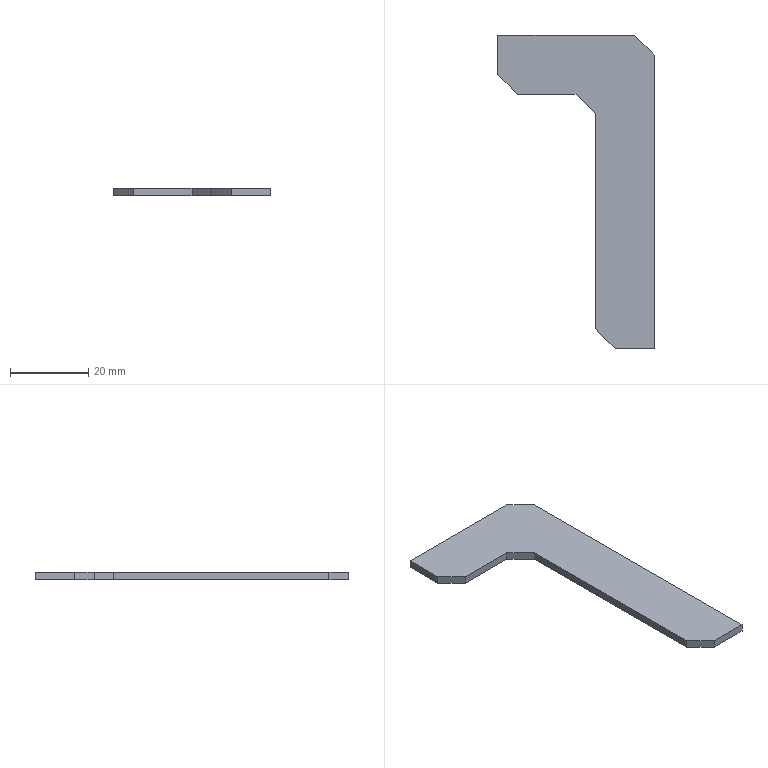Part | STEP file | SynoNew-0304-056 | 1 solid | 12 faces | box 40 x 80 x 2 mm | volume 3100 mm3 | plane 12
STEP:
#1=CARTESIAN_POINT('',(-15.,25.,2.));
#2=VERTEX_POINT('',#1);
#3=CARTESIAN_POINT('',(-20.,30.,2.));
#4=VERTEX_POINT('',#3);
#5=CARTESIAN_POINT('',(-6.25,16.25,2.));
#6=DIRECTION('',(-0.7071,0.7071,0.));
#7=VECTOR('',#6,10.);
#8=LINE('',#5,#7);
#9=EDGE_CURVE('',#2,#4,#8,.T.);
#10=ORIENTED_EDGE('',*,*,#9,.T.);
#11=CARTESIAN_POINT('',(-20.,30.,0.));
#12=VERTEX_POINT('',#11);
#13=CARTESIAN_POINT('',(-20.,30.,1.));
#14=DIRECTION('',(0.,0.,-1.));
#15=VECTOR('',#14,10.);
#16=LINE('',#13,#15);
#17=EDGE_CURVE('',#4,#12,#16,.T.);
#18=ORIENTED_EDGE('',*,*,#17,.T.);
#19=CARTESIAN_POINT('',(-15.,25.,0.));
#20=VERTEX_POINT('',#19);
#21=CARTESIAN_POINT('',(-6.25,16.25,0.));
#22=DIRECTION('',(0.7071,-0.7071,0.));
#23=VECTOR('',#22,10.);
#24=LINE('',#21,#23);
#25=EDGE_CURVE('',#12,#20,#24,.T.);
#26=ORIENTED_EDGE('',*,*,#25,.T.);
#27=CARTESIAN_POINT('',(-15.,25.,1.));
#28=DIRECTION('',(0.,0.,1.));
#29=VECTOR('',#28,10.);
#30=LINE('',#27,#29);
#31=EDGE_CURVE('',#20,#2,#30,.T.);
#32=ORIENTED_EDGE('',*,*,#31,.T.);
#33=EDGE_LOOP('',(#10,#18,#26,#32));
#34=FACE_OUTER_BOUND('',#33,.T.);
#35=CARTESIAN_POINT('',(-17.5,27.5,1.));
#36=DIRECTION('',(-0.7071,-0.7071,0.));
#37=DIRECTION('',(0.,0.,1.));
#38=AXIS2_PLACEMENT_3D('',#35,#36,#37);
#39=PLANE('',#38);
#40=ADVANCED_FACE('',(#34),#39,.T.);
#41=ORIENTED_EDGE('',*,*,#31,.F.);
#42=CARTESIAN_POINT('',(0.,25.,0.));
#43=VERTEX_POINT('',#42);
#44=CARTESIAN_POINT('',(-16.04,25.,0.));
#45=DIRECTION('',(-1.,0.,0.));
#46=VECTOR('',#45,10.);
#47=LINE('',#44,#46);
#48=EDGE_CURVE('',#43,#20,#47,.T.);
#49=ORIENTED_EDGE('',*,*,#48,.F.);
#50=CARTESIAN_POINT('',(0.,25.,2.));
#51=VERTEX_POINT('',#50);
#52=CARTESIAN_POINT('',(0.,25.,2.));
#53=DIRECTION('',(0.,0.,-1.));
#54=VECTOR('',#53,10.);
#55=LINE('',#52,#54);
#56=EDGE_CURVE('',#51,#43,#55,.T.);
#57=ORIENTED_EDGE('',*,*,#56,.F.);
#58=CARTESIAN_POINT('',(-16.04,25.,2.));
#59=DIRECTION('',(1.,0.,0.));
#60=VECTOR('',#59,10.);
#61=LINE('',#58,#60);
#62=EDGE_CURVE('',#2,#51,#61,.T.);
#63=ORIENTED_EDGE('',*,*,#62,.F.);
#64=EDGE_LOOP('',(#41,#49,#57,#63));
#65=FACE_OUTER_BOUND('',#64,.T.);
#66=CARTESIAN_POINT('',(-32.08,25.,2.));
#67=DIRECTION('',(0.,1.,0.));
#68=DIRECTION('',(1.,0.,0.));
#69=AXIS2_PLACEMENT_3D('',#66,#67,#68);
#70=PLANE('',#69);
#71=ADVANCED_FACE('',(#65),#70,.F.);
#72=ORIENTED_EDGE('',*,*,#25,.F.);
#73=CARTESIAN_POINT('',(-20.,40.,0.));
#74=VERTEX_POINT('',#73);
#75=CARTESIAN_POINT('',(-20.,40.,0.));
#76=DIRECTION('',(0.,-1.,0.));
#77=VECTOR('',#76,10.);
#78=LINE('',#75,#77);
#79=EDGE_CURVE('',#74,#12,#78,.T.);
#80=ORIENTED_EDGE('',*,*,#79,.F.);
#81=CARTESIAN_POINT('',(15.,40.,0.));
#82=VERTEX_POINT('',#81);
#83=CARTESIAN_POINT('',(20.,40.,0.));
#84=DIRECTION('',(-1.,0.,0.));
#85=VECTOR('',#84,10.);
#86=LINE('',#83,#85);
#87=EDGE_CURVE('',#82,#74,#86,.T.);
#88=ORIENTED_EDGE('',*,*,#87,.F.);
#89=CARTESIAN_POINT('',(20.,35.,0.));
#90=VERTEX_POINT('',#89);
#91=CARTESIAN_POINT('',(22.5,32.5,0.));
#92=DIRECTION('',(-0.7071,0.7071,0.));
#93=VECTOR('',#92,10.);
#94=LINE('',#91,#93);
#95=EDGE_CURVE('',#90,#82,#94,.T.);
#96=ORIENTED_EDGE('',*,*,#95,.F.);
#97=CARTESIAN_POINT('',(20.,-40.,0.));
#98=VERTEX_POINT('',#97);
#99=CARTESIAN_POINT('',(20.,-40.,0.));
#100=DIRECTION('',(0.,1.,0.));
#101=VECTOR('',#100,10.);
#102=LINE('',#99,#101);
#103=EDGE_CURVE('',#98,#90,#102,.T.);
#104=ORIENTED_EDGE('',*,*,#103,.F.);
#105=CARTESIAN_POINT('',(10.,-40.,0.));
#106=VERTEX_POINT('',#105);
#107=CARTESIAN_POINT('',(-20.,-40.,0.));
#108=DIRECTION('',(1.,0.,0.));
#109=VECTOR('',#108,10.);
#110=LINE('',#107,#109);
#111=EDGE_CURVE('',#106,#98,#110,.T.);
#112=ORIENTED_EDGE('',*,*,#111,.F.);
#113=CARTESIAN_POINT('',(5.,-35.,0.));
#114=VERTEX_POINT('',#113);
#115=CARTESIAN_POINT('',(-3.75,-26.25,0.));
#116=DIRECTION('',(0.7071,-0.7071,0.));
#117=VECTOR('',#116,10.);
#118=LINE('',#115,#117);
#119=EDGE_CURVE('',#114,#106,#118,.T.);
#120=ORIENTED_EDGE('',*,*,#119,.F.);
#121=CARTESIAN_POINT('',(5.,20.,0.));
#122=VERTEX_POINT('',#121);
#123=CARTESIAN_POINT('',(5.,12.5,0.));
#124=DIRECTION('',(0.,1.,0.));
#125=VECTOR('',#124,10.);
#126=LINE('',#123,#125);
#127=EDGE_CURVE('',#114,#122,#126,.T.);
#128=ORIENTED_EDGE('',*,*,#127,.T.);
#129=CARTESIAN_POINT('',(7.5,17.5,0.));
#130=DIRECTION('',(0.7071,-0.7071,0.));
#131=VECTOR('',#130,10.);
#132=LINE('',#129,#131);
#133=EDGE_CURVE('',#43,#122,#132,.T.);
#134=ORIENTED_EDGE('',*,*,#133,.F.);
#135=ORIENTED_EDGE('',*,*,#48,.T.);
#136=EDGE_LOOP('',(#72,#80,#88,#96,#104,#112,#120,#128,#134,#135));
#137=FACE_OUTER_BOUND('',#136,.T.);
#138=CARTESIAN_POINT('',(0.,0.,0.));
#139=DIRECTION('',(0.,0.,1.));
#140=DIRECTION('',(1.,0.,0.));
#141=AXIS2_PLACEMENT_3D('',#138,#139,#140);
#142=PLANE('',#141);
#143=ADVANCED_FACE('',(#137),#142,.F.);
#144=ORIENTED_EDGE('',*,*,#119,.T.);
#145=CARTESIAN_POINT('',(10.,-40.,2.));
#146=VERTEX_POINT('',#145);
#147=CARTESIAN_POINT('',(10.,-40.,1.));
#148=DIRECTION('',(0.,0.,1.));
#149=VECTOR('',#148,10.);
#150=LINE('',#147,#149);
#151=EDGE_CURVE('',#106,#146,#150,.T.);
#152=ORIENTED_EDGE('',*,*,#151,.T.);
#153=CARTESIAN_POINT('',(5.,-35.,2.));
#154=VERTEX_POINT('',#153);
#155=CARTESIAN_POINT('',(-3.75,-26.25,2.));
#156=DIRECTION('',(-0.7071,0.7071,0.));
#157=VECTOR('',#156,10.);
#158=LINE('',#155,#157);
#159=EDGE_CURVE('',#146,#154,#158,.T.);
#160=ORIENTED_EDGE('',*,*,#159,.T.);
#161=CARTESIAN_POINT('',(5.,-35.,1.));
#162=DIRECTION('',(0.,0.,-1.));
#163=VECTOR('',#162,10.);
#164=LINE('',#161,#163);
#165=EDGE_CURVE('',#154,#114,#164,.T.);
#166=ORIENTED_EDGE('',*,*,#165,.T.);
#167=EDGE_LOOP('',(#144,#152,#160,#166));
#168=FACE_OUTER_BOUND('',#167,.T.);
#169=CARTESIAN_POINT('',(7.5,-37.5,1.));
#170=DIRECTION('',(-0.7071,-0.7071,0.));
#171=DIRECTION('',(0.,0.,1.));
#172=AXIS2_PLACEMENT_3D('',#169,#170,#171);
#173=PLANE('',#172);
#174=ADVANCED_FACE('',(#168),#173,.T.);
#175=ORIENTED_EDGE('',*,*,#165,.F.);
#176=CARTESIAN_POINT('',(5.,20.,2.));
#177=VERTEX_POINT('',#176);
#178=CARTESIAN_POINT('',(5.,12.5,2.));
#179=DIRECTION('',(0.,-1.,0.));
#180=VECTOR('',#179,10.);
#181=LINE('',#178,#180);
#182=EDGE_CURVE('',#177,#154,#181,.T.);
#183=ORIENTED_EDGE('',*,*,#182,.F.);
#184=CARTESIAN_POINT('',(5.,20.,2.));
#185=DIRECTION('',(0.,0.,1.));
#186=VECTOR('',#185,10.);
#187=LINE('',#184,#186);
#188=EDGE_CURVE('',#122,#177,#187,.T.);
#189=ORIENTED_EDGE('',*,*,#188,.F.);
#190=ORIENTED_EDGE('',*,*,#127,.F.);
#191=EDGE_LOOP('',(#175,#183,#189,#190));
#192=FACE_OUTER_BOUND('',#191,.T.);
#193=CARTESIAN_POINT('',(5.,25.,2.));
#194=DIRECTION('',(1.,0.,0.));
#195=DIRECTION('',(0.,-1.,0.));
#196=AXIS2_PLACEMENT_3D('',#193,#194,#195);
#197=PLANE('',#196);
#198=ADVANCED_FACE('',(#192),#197,.F.);
#199=CARTESIAN_POINT('',(7.5,17.5,2.));
#200=DIRECTION('',(-0.7071,0.7071,0.));
#201=VECTOR('',#200,10.);
#202=LINE('',#199,#201);
#203=EDGE_CURVE('',#177,#51,#202,.T.);
#204=ORIENTED_EDGE('',*,*,#203,.T.);
#205=ORIENTED_EDGE('',*,*,#56,.T.);
#206=ORIENTED_EDGE('',*,*,#133,.T.);
#207=ORIENTED_EDGE('',*,*,#188,.T.);
#208=EDGE_LOOP('',(#204,#205,#206,#207));
#209=FACE_OUTER_BOUND('',#208,.T.);
#210=CARTESIAN_POINT('',(2.5,22.5,2.));
#211=DIRECTION('',(-0.7071,-0.7071,0.));
#212=DIRECTION('',(0.,0.,1.));
#213=AXIS2_PLACEMENT_3D('',#210,#211,#212);
#214=PLANE('',#213);
#215=ADVANCED_FACE('',(#209),#214,.T.);
#216=ORIENTED_EDGE('',*,*,#17,.F.);
#217=CARTESIAN_POINT('',(-20.,40.,2.));
#218=VERTEX_POINT('',#217);
#219=CARTESIAN_POINT('',(-20.,40.,2.));
#220=DIRECTION('',(0.,-1.,0.));
#221=VECTOR('',#220,10.);
#222=LINE('',#219,#221);
#223=EDGE_CURVE('',#218,#4,#222,.T.);
#224=ORIENTED_EDGE('',*,*,#223,.F.);
#225=CARTESIAN_POINT('',(-20.,40.,0.));
#226=DIRECTION('',(0.,0.,1.));
#227=VECTOR('',#226,10.);
#228=LINE('',#225,#227);
#229=EDGE_CURVE('',#74,#218,#228,.T.);
#230=ORIENTED_EDGE('',*,*,#229,.F.);
#231=ORIENTED_EDGE('',*,*,#79,.T.);
#232=EDGE_LOOP('',(#216,#224,#230,#231));
#233=FACE_OUTER_BOUND('',#232,.T.);
#234=CARTESIAN_POINT('',(-20.,40.,0.));
#235=DIRECTION('',(-1.,0.,0.));
#236=DIRECTION('',(0.,-1.,0.));
#237=AXIS2_PLACEMENT_3D('',#234,#235,#236);
#238=PLANE('',#237);
#239=ADVANCED_FACE('',(#233),#238,.T.);
#240=ORIENTED_EDGE('',*,*,#9,.F.);
#241=ORIENTED_EDGE('',*,*,#62,.T.);
#242=ORIENTED_EDGE('',*,*,#203,.F.);
#243=ORIENTED_EDGE('',*,*,#182,.T.);
#244=ORIENTED_EDGE('',*,*,#159,.F.);
#245=CARTESIAN_POINT('',(20.,-40.,2.));
#246=VERTEX_POINT('',#245);
#247=CARTESIAN_POINT('',(-20.,-40.,2.));
#248=DIRECTION('',(1.,0.,0.));
#249=VECTOR('',#248,10.);
#250=LINE('',#247,#249);
#251=EDGE_CURVE('',#146,#246,#250,.T.);
#252=ORIENTED_EDGE('',*,*,#251,.T.);
#253=CARTESIAN_POINT('',(20.,35.,2.));
#254=VERTEX_POINT('',#253);
#255=CARTESIAN_POINT('',(20.,-40.,2.));
#256=DIRECTION('',(0.,1.,0.));
#257=VECTOR('',#256,10.);
#258=LINE('',#255,#257);
#259=EDGE_CURVE('',#246,#254,#258,.T.);
#260=ORIENTED_EDGE('',*,*,#259,.T.);
#261=CARTESIAN_POINT('',(15.,40.,2.));
#262=VERTEX_POINT('',#261);
#263=CARTESIAN_POINT('',(22.5,32.5,2.));
#264=DIRECTION('',(0.7071,-0.7071,0.));
#265=VECTOR('',#264,10.);
#266=LINE('',#263,#265);
#267=EDGE_CURVE('',#262,#254,#266,.T.);
#268=ORIENTED_EDGE('',*,*,#267,.F.);
#269=CARTESIAN_POINT('',(20.,40.,2.));
#270=DIRECTION('',(-1.,0.,0.));
#271=VECTOR('',#270,10.);
#272=LINE('',#269,#271);
#273=EDGE_CURVE('',#262,#218,#272,.T.);
#274=ORIENTED_EDGE('',*,*,#273,.T.);
#275=ORIENTED_EDGE('',*,*,#223,.T.);
#276=EDGE_LOOP('',(#240,#241,#242,#243,#244,#252,#260,#268,#274,#275));
#277=FACE_OUTER_BOUND('',#276,.T.);
#278=CARTESIAN_POINT('',(0.,0.,2.));
#279=DIRECTION('',(0.,0.,1.));
#280=DIRECTION('',(1.,0.,0.));
#281=AXIS2_PLACEMENT_3D('',#278,#279,#280);
#282=PLANE('',#281);
#283=ADVANCED_FACE('',(#277),#282,.T.);
#284=ORIENTED_EDGE('',*,*,#267,.T.);
#285=CARTESIAN_POINT('',(20.,35.,0.));
#286=DIRECTION('',(0.,0.,-1.));
#287=VECTOR('',#286,10.);
#288=LINE('',#285,#287);
#289=EDGE_CURVE('',#254,#90,#288,.T.);
#290=ORIENTED_EDGE('',*,*,#289,.T.);
#291=ORIENTED_EDGE('',*,*,#95,.T.);
#292=CARTESIAN_POINT('',(15.,40.,0.));
#293=DIRECTION('',(0.,0.,1.));
#294=VECTOR('',#293,10.);
#295=LINE('',#292,#294);
#296=EDGE_CURVE('',#82,#262,#295,.T.);
#297=ORIENTED_EDGE('',*,*,#296,.T.);
#298=EDGE_LOOP('',(#284,#290,#291,#297));
#299=FACE_OUTER_BOUND('',#298,.T.);
#300=CARTESIAN_POINT('',(17.5,37.5,0.));
#301=DIRECTION('',(0.7071,0.7071,0.));
#302=DIRECTION('',(0.,0.,-1.));
#303=AXIS2_PLACEMENT_3D('',#300,#301,#302);
#304=PLANE('',#303);
#305=ADVANCED_FACE('',(#299),#304,.T.);
#306=ORIENTED_EDGE('',*,*,#296,.F.);
#307=ORIENTED_EDGE('',*,*,#87,.T.);
#308=ORIENTED_EDGE('',*,*,#229,.T.);
#309=ORIENTED_EDGE('',*,*,#273,.F.);
#310=EDGE_LOOP('',(#306,#307,#308,#309));
#311=FACE_OUTER_BOUND('',#310,.T.);
#312=CARTESIAN_POINT('',(20.,40.,0.));
#313=DIRECTION('',(0.,1.,0.));
#314=DIRECTION('',(-1.,0.,0.));
#315=AXIS2_PLACEMENT_3D('',#312,#313,#314);
#316=PLANE('',#315);
#317=ADVANCED_FACE('',(#311),#316,.T.);
#318=ORIENTED_EDGE('',*,*,#289,.F.);
#319=ORIENTED_EDGE('',*,*,#259,.F.);
#320=CARTESIAN_POINT('',(20.,-40.,0.));
#321=DIRECTION('',(0.,0.,1.));
#322=VECTOR('',#321,10.);
#323=LINE('',#320,#322);
#324=EDGE_CURVE('',#98,#246,#323,.T.);
#325=ORIENTED_EDGE('',*,*,#324,.F.);
#326=ORIENTED_EDGE('',*,*,#103,.T.);
#327=EDGE_LOOP('',(#318,#319,#325,#326));
#328=FACE_OUTER_BOUND('',#327,.T.);
#329=CARTESIAN_POINT('',(20.,-40.,0.));
#330=DIRECTION('',(1.,0.,0.));
#331=DIRECTION('',(0.,1.,0.));
#332=AXIS2_PLACEMENT_3D('',#329,#330,#331);
#333=PLANE('',#332);
#334=ADVANCED_FACE('',(#328),#333,.T.);
#335=ORIENTED_EDGE('',*,*,#151,.F.);
#336=ORIENTED_EDGE('',*,*,#111,.T.);
#337=ORIENTED_EDGE('',*,*,#324,.T.);
#338=ORIENTED_EDGE('',*,*,#251,.F.);
#339=EDGE_LOOP('',(#335,#336,#337,#338));
#340=FACE_OUTER_BOUND('',#339,.T.);
#341=CARTESIAN_POINT('',(-20.,-40.,0.));
#342=DIRECTION('',(0.,-1.,0.));
#343=DIRECTION('',(1.,0.,0.));
#344=AXIS2_PLACEMENT_3D('',#341,#342,#343);
#345=PLANE('',#344);
#346=ADVANCED_FACE('',(#340),#345,.T.);
#347=CLOSED_SHELL('',(#40,#71,#143,#174,#198,#215,#239,#283,#305,#317,#334,#346));
#348=MANIFOLD_SOLID_BREP('',#347);
#349=(LENGTH_UNIT()NAMED_UNIT(*)SI_UNIT(.MILLI.,.METRE.));
#350=UNCERTAINTY_MEASURE_WITH_UNIT(LENGTH_MEASURE(0.01),#349,'','');
#351=(NAMED_UNIT(*)PLANE_ANGLE_UNIT()SI_UNIT($,.RADIAN.));
#352=(NAMED_UNIT(*)SI_UNIT($,.STERADIAN.)SOLID_ANGLE_UNIT());
#353=(GEOMETRIC_REPRESENTATION_CONTEXT(3)GLOBAL_UNCERTAINTY_ASSIGNED_CONTEXT((#350))GLOBAL_UNIT_ASSIGNED_CONTEXT((#349,#351,#352))REPRESENTATION_CONTEXT('',''));
#354=ADVANCED_BREP_SHAPE_REPRESENTATION('',(#348),#353);